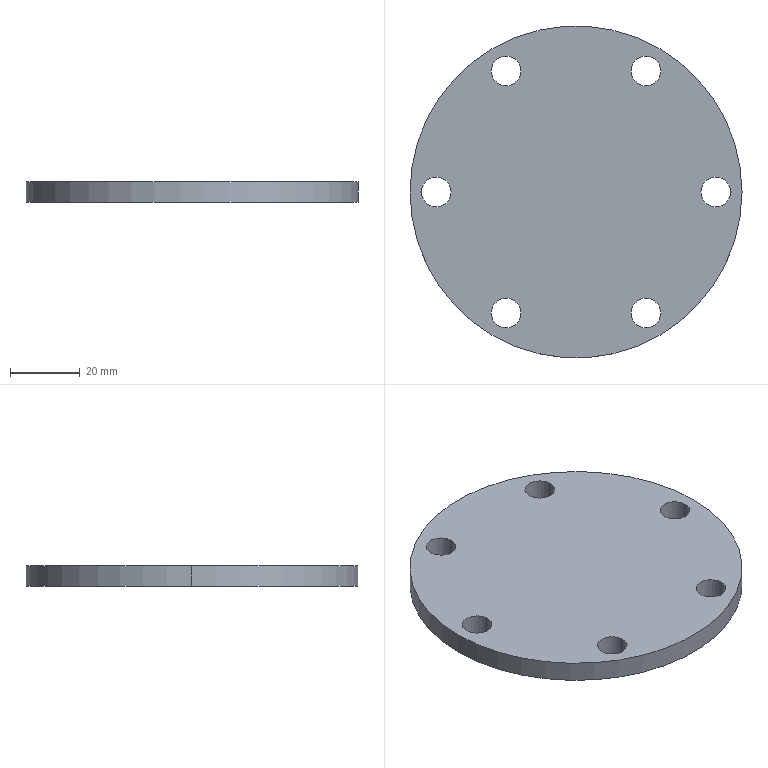Part | SolidWorks | features FlatPattern 1, SMBaseFlange 1, SheetMetal 1 | 1 solid | 16 faces | box 95 x 95 x 6 mm | volume 40486 mm3 | cylinder 14 | plane 2 | commonest cylinder face diameters 8.5 x12 95 x2
STEP:
#1=CARTESIAN_POINT('',(15.75,-34.641,6.));
#2=VERTEX_POINT('',#1);
#3=CARTESIAN_POINT('',(24.25,-34.641,6.));
#4=VERTEX_POINT('',#3);
#5=CARTESIAN_POINT('',(20.,-34.641,6.));
#6=DIRECTION('',(0.,0.,1.));
#7=DIRECTION('',(1.,0.,0.));
#8=AXIS2_PLACEMENT_3D('',#5,#6,#7);
#9=CIRCLE('',#8,4.25);
#10=EDGE_CURVE('',#2,#4,#9,.T.);
#11=ORIENTED_EDGE('',*,*,#10,.T.);
#12=CARTESIAN_POINT('',(24.25,-34.641,0.));
#13=VERTEX_POINT('',#12);
#14=CARTESIAN_POINT('',(24.25,-34.641,6.));
#15=DIRECTION('',(0.,0.,-1.));
#16=VECTOR('',#15,1000.);
#17=LINE('',#14,#16);
#18=EDGE_CURVE('',#4,#13,#17,.T.);
#19=ORIENTED_EDGE('',*,*,#18,.T.);
#20=CARTESIAN_POINT('',(15.75,-34.641,0.));
#21=VERTEX_POINT('',#20);
#22=CARTESIAN_POINT('',(20.,-34.641,0.));
#23=DIRECTION('',(0.,0.,1.));
#24=DIRECTION('',(1.,0.,0.));
#25=AXIS2_PLACEMENT_3D('',#22,#23,#24);
#26=CIRCLE('',#25,4.25);
#27=EDGE_CURVE('',#21,#13,#26,.T.);
#28=ORIENTED_EDGE('',*,*,#27,.F.);
#29=CARTESIAN_POINT('',(15.75,-34.641,6.));
#30=DIRECTION('',(0.,0.,-1.));
#31=VECTOR('',#30,1000.);
#32=LINE('',#29,#31);
#33=EDGE_CURVE('',#2,#21,#32,.T.);
#34=ORIENTED_EDGE('',*,*,#33,.F.);
#35=EDGE_LOOP('',(#11,#19,#28,#34));
#36=FACE_OUTER_BOUND('',#35,.T.);
#37=CARTESIAN_POINT('',(20.,-34.641,6.));
#38=DIRECTION('',(0.,0.,-1.));
#39=DIRECTION('',(-1.,0.,0.));
#40=AXIS2_PLACEMENT_3D('',#37,#38,#39);
#41=CYLINDRICAL_SURFACE('',#40,4.25);
#42=ADVANCED_FACE('',(#36),#41,.F.);
#43=CARTESIAN_POINT('',(35.75,0.,6.));
#44=VERTEX_POINT('',#43);
#45=CARTESIAN_POINT('',(44.25,0.,6.));
#46=VERTEX_POINT('',#45);
#47=CARTESIAN_POINT('',(40.,0.,6.));
#48=DIRECTION('',(0.,0.,1.));
#49=DIRECTION('',(1.,0.,0.));
#50=AXIS2_PLACEMENT_3D('',#47,#48,#49);
#51=CIRCLE('',#50,4.25);
#52=EDGE_CURVE('',#44,#46,#51,.T.);
#53=ORIENTED_EDGE('',*,*,#52,.T.);
#54=CARTESIAN_POINT('',(44.25,0.,0.));
#55=VERTEX_POINT('',#54);
#56=CARTESIAN_POINT('',(44.25,0.,6.));
#57=DIRECTION('',(0.,0.,-1.));
#58=VECTOR('',#57,1000.);
#59=LINE('',#56,#58);
#60=EDGE_CURVE('',#46,#55,#59,.T.);
#61=ORIENTED_EDGE('',*,*,#60,.T.);
#62=CARTESIAN_POINT('',(35.75,0.,0.));
#63=VERTEX_POINT('',#62);
#64=CARTESIAN_POINT('',(40.,0.,0.));
#65=DIRECTION('',(0.,0.,1.));
#66=DIRECTION('',(1.,0.,0.));
#67=AXIS2_PLACEMENT_3D('',#64,#65,#66);
#68=CIRCLE('',#67,4.25);
#69=EDGE_CURVE('',#63,#55,#68,.T.);
#70=ORIENTED_EDGE('',*,*,#69,.F.);
#71=CARTESIAN_POINT('',(35.75,0.,6.));
#72=DIRECTION('',(0.,0.,-1.));
#73=VECTOR('',#72,1000.);
#74=LINE('',#71,#73);
#75=EDGE_CURVE('',#44,#63,#74,.T.);
#76=ORIENTED_EDGE('',*,*,#75,.F.);
#77=EDGE_LOOP('',(#53,#61,#70,#76));
#78=FACE_OUTER_BOUND('',#77,.T.);
#79=CARTESIAN_POINT('',(40.,0.,6.));
#80=DIRECTION('',(0.,0.,-1.));
#81=DIRECTION('',(-1.,0.,0.));
#82=AXIS2_PLACEMENT_3D('',#79,#80,#81);
#83=CYLINDRICAL_SURFACE('',#82,4.25);
#84=ADVANCED_FACE('',(#78),#83,.F.);
#85=CARTESIAN_POINT('',(15.75,34.641,6.));
#86=VERTEX_POINT('',#85);
#87=CARTESIAN_POINT('',(24.25,34.641,6.));
#88=VERTEX_POINT('',#87);
#89=CARTESIAN_POINT('',(20.,34.641,6.));
#90=DIRECTION('',(0.,0.,1.));
#91=DIRECTION('',(1.,0.,0.));
#92=AXIS2_PLACEMENT_3D('',#89,#90,#91);
#93=CIRCLE('',#92,4.25);
#94=EDGE_CURVE('',#86,#88,#93,.T.);
#95=ORIENTED_EDGE('',*,*,#94,.T.);
#96=CARTESIAN_POINT('',(24.25,34.641,0.));
#97=VERTEX_POINT('',#96);
#98=CARTESIAN_POINT('',(24.25,34.641,6.));
#99=DIRECTION('',(0.,0.,-1.));
#100=VECTOR('',#99,1000.);
#101=LINE('',#98,#100);
#102=EDGE_CURVE('',#88,#97,#101,.T.);
#103=ORIENTED_EDGE('',*,*,#102,.T.);
#104=CARTESIAN_POINT('',(15.75,34.641,0.));
#105=VERTEX_POINT('',#104);
#106=CARTESIAN_POINT('',(20.,34.641,0.));
#107=DIRECTION('',(0.,0.,1.));
#108=DIRECTION('',(1.,0.,0.));
#109=AXIS2_PLACEMENT_3D('',#106,#107,#108);
#110=CIRCLE('',#109,4.25);
#111=EDGE_CURVE('',#105,#97,#110,.T.);
#112=ORIENTED_EDGE('',*,*,#111,.F.);
#113=CARTESIAN_POINT('',(15.75,34.641,6.));
#114=DIRECTION('',(0.,0.,-1.));
#115=VECTOR('',#114,1000.);
#116=LINE('',#113,#115);
#117=EDGE_CURVE('',#86,#105,#116,.T.);
#118=ORIENTED_EDGE('',*,*,#117,.F.);
#119=EDGE_LOOP('',(#95,#103,#112,#118));
#120=FACE_OUTER_BOUND('',#119,.T.);
#121=CARTESIAN_POINT('',(20.,34.641,6.));
#122=DIRECTION('',(0.,0.,-1.));
#123=DIRECTION('',(-1.,0.,0.));
#124=AXIS2_PLACEMENT_3D('',#121,#122,#123);
#125=CYLINDRICAL_SURFACE('',#124,4.25);
#126=ADVANCED_FACE('',(#120),#125,.F.);
#127=CARTESIAN_POINT('',(-24.25,34.641,6.));
#128=VERTEX_POINT('',#127);
#129=CARTESIAN_POINT('',(-15.75,34.641,6.));
#130=VERTEX_POINT('',#129);
#131=CARTESIAN_POINT('',(-20.,34.641,6.));
#132=DIRECTION('',(0.,0.,1.));
#133=DIRECTION('',(1.,0.,0.));
#134=AXIS2_PLACEMENT_3D('',#131,#132,#133);
#135=CIRCLE('',#134,4.25);
#136=EDGE_CURVE('',#128,#130,#135,.T.);
#137=ORIENTED_EDGE('',*,*,#136,.T.);
#138=CARTESIAN_POINT('',(-15.75,34.641,0.));
#139=VERTEX_POINT('',#138);
#140=CARTESIAN_POINT('',(-15.75,34.641,6.));
#141=DIRECTION('',(0.,0.,-1.));
#142=VECTOR('',#141,1000.);
#143=LINE('',#140,#142);
#144=EDGE_CURVE('',#130,#139,#143,.T.);
#145=ORIENTED_EDGE('',*,*,#144,.T.);
#146=CARTESIAN_POINT('',(-24.25,34.641,0.));
#147=VERTEX_POINT('',#146);
#148=CARTESIAN_POINT('',(-20.,34.641,0.));
#149=DIRECTION('',(0.,0.,1.));
#150=DIRECTION('',(1.,0.,0.));
#151=AXIS2_PLACEMENT_3D('',#148,#149,#150);
#152=CIRCLE('',#151,4.25);
#153=EDGE_CURVE('',#147,#139,#152,.T.);
#154=ORIENTED_EDGE('',*,*,#153,.F.);
#155=CARTESIAN_POINT('',(-24.25,34.641,6.));
#156=DIRECTION('',(0.,0.,-1.));
#157=VECTOR('',#156,1000.);
#158=LINE('',#155,#157);
#159=EDGE_CURVE('',#128,#147,#158,.T.);
#160=ORIENTED_EDGE('',*,*,#159,.F.);
#161=EDGE_LOOP('',(#137,#145,#154,#160));
#162=FACE_OUTER_BOUND('',#161,.T.);
#163=CARTESIAN_POINT('',(-20.,34.641,6.));
#164=DIRECTION('',(0.,0.,-1.));
#165=DIRECTION('',(-1.,0.,0.));
#166=AXIS2_PLACEMENT_3D('',#163,#164,#165);
#167=CYLINDRICAL_SURFACE('',#166,4.25);
#168=ADVANCED_FACE('',(#162),#167,.F.);
#169=CARTESIAN_POINT('',(-44.25,0.,6.));
#170=VERTEX_POINT('',#169);
#171=CARTESIAN_POINT('',(-35.75,0.,6.));
#172=VERTEX_POINT('',#171);
#173=CARTESIAN_POINT('',(-40.,0.,6.));
#174=DIRECTION('',(0.,0.,1.));
#175=DIRECTION('',(1.,0.,0.));
#176=AXIS2_PLACEMENT_3D('',#173,#174,#175);
#177=CIRCLE('',#176,4.25);
#178=EDGE_CURVE('',#170,#172,#177,.T.);
#179=ORIENTED_EDGE('',*,*,#178,.T.);
#180=CARTESIAN_POINT('',(-35.75,0.,0.));
#181=VERTEX_POINT('',#180);
#182=CARTESIAN_POINT('',(-35.75,0.,6.));
#183=DIRECTION('',(0.,0.,-1.));
#184=VECTOR('',#183,1000.);
#185=LINE('',#182,#184);
#186=EDGE_CURVE('',#172,#181,#185,.T.);
#187=ORIENTED_EDGE('',*,*,#186,.T.);
#188=CARTESIAN_POINT('',(-44.25,0.,0.));
#189=VERTEX_POINT('',#188);
#190=CARTESIAN_POINT('',(-40.,0.,0.));
#191=DIRECTION('',(0.,0.,1.));
#192=DIRECTION('',(1.,0.,0.));
#193=AXIS2_PLACEMENT_3D('',#190,#191,#192);
#194=CIRCLE('',#193,4.25);
#195=EDGE_CURVE('',#189,#181,#194,.T.);
#196=ORIENTED_EDGE('',*,*,#195,.F.);
#197=CARTESIAN_POINT('',(-44.25,0.,6.));
#198=DIRECTION('',(0.,0.,-1.));
#199=VECTOR('',#198,1000.);
#200=LINE('',#197,#199);
#201=EDGE_CURVE('',#170,#189,#200,.T.);
#202=ORIENTED_EDGE('',*,*,#201,.F.);
#203=EDGE_LOOP('',(#179,#187,#196,#202));
#204=FACE_OUTER_BOUND('',#203,.T.);
#205=CARTESIAN_POINT('',(-40.,0.,6.));
#206=DIRECTION('',(0.,0.,-1.));
#207=DIRECTION('',(-1.,0.,0.));
#208=AXIS2_PLACEMENT_3D('',#205,#206,#207);
#209=CYLINDRICAL_SURFACE('',#208,4.25);
#210=ADVANCED_FACE('',(#204),#209,.F.);
#211=CARTESIAN_POINT('',(-24.25,-34.641,6.));
#212=VERTEX_POINT('',#211);
#213=CARTESIAN_POINT('',(-15.75,-34.641,6.));
#214=VERTEX_POINT('',#213);
#215=CARTESIAN_POINT('',(-20.,-34.641,6.));
#216=DIRECTION('',(0.,0.,1.));
#217=DIRECTION('',(1.,0.,0.));
#218=AXIS2_PLACEMENT_3D('',#215,#216,#217);
#219=CIRCLE('',#218,4.25);
#220=EDGE_CURVE('',#212,#214,#219,.T.);
#221=ORIENTED_EDGE('',*,*,#220,.T.);
#222=CARTESIAN_POINT('',(-15.75,-34.641,0.));
#223=VERTEX_POINT('',#222);
#224=CARTESIAN_POINT('',(-15.75,-34.641,6.));
#225=DIRECTION('',(0.,0.,-1.));
#226=VECTOR('',#225,1000.);
#227=LINE('',#224,#226);
#228=EDGE_CURVE('',#214,#223,#227,.T.);
#229=ORIENTED_EDGE('',*,*,#228,.T.);
#230=CARTESIAN_POINT('',(-24.25,-34.641,0.));
#231=VERTEX_POINT('',#230);
#232=CARTESIAN_POINT('',(-20.,-34.641,0.));
#233=DIRECTION('',(0.,0.,1.));
#234=DIRECTION('',(1.,0.,0.));
#235=AXIS2_PLACEMENT_3D('',#232,#233,#234);
#236=CIRCLE('',#235,4.25);
#237=EDGE_CURVE('',#231,#223,#236,.T.);
#238=ORIENTED_EDGE('',*,*,#237,.F.);
#239=CARTESIAN_POINT('',(-24.25,-34.641,6.));
#240=DIRECTION('',(0.,0.,-1.));
#241=VECTOR('',#240,1000.);
#242=LINE('',#239,#241);
#243=EDGE_CURVE('',#212,#231,#242,.T.);
#244=ORIENTED_EDGE('',*,*,#243,.F.);
#245=EDGE_LOOP('',(#221,#229,#238,#244));
#246=FACE_OUTER_BOUND('',#245,.T.);
#247=CARTESIAN_POINT('',(-20.,-34.641,6.));
#248=DIRECTION('',(0.,0.,-1.));
#249=DIRECTION('',(-1.,0.,0.));
#250=AXIS2_PLACEMENT_3D('',#247,#248,#249);
#251=CYLINDRICAL_SURFACE('',#250,4.25);
#252=ADVANCED_FACE('',(#246),#251,.F.);
#253=CARTESIAN_POINT('',(47.5,0.,6.));
#254=VERTEX_POINT('',#253);
#255=CARTESIAN_POINT('',(-47.5,0.,6.));
#256=VERTEX_POINT('',#255);
#257=CARTESIAN_POINT('',(0.,0.,6.));
#258=DIRECTION('',(0.,0.,1.));
#259=DIRECTION('',(1.,0.,0.));
#260=AXIS2_PLACEMENT_3D('',#257,#258,#259);
#261=CIRCLE('',#260,47.5);
#262=EDGE_CURVE('',#254,#256,#261,.T.);
#263=ORIENTED_EDGE('',*,*,#262,.F.);
#264=CARTESIAN_POINT('',(47.5,0.,0.));
#265=VERTEX_POINT('',#264);
#266=CARTESIAN_POINT('',(47.5,0.,6.));
#267=DIRECTION('',(0.,0.,-1.));
#268=VECTOR('',#267,1000.);
#269=LINE('',#266,#268);
#270=EDGE_CURVE('',#254,#265,#269,.T.);
#271=ORIENTED_EDGE('',*,*,#270,.T.);
#272=CARTESIAN_POINT('',(-47.5,0.,0.));
#273=VERTEX_POINT('',#272);
#274=CARTESIAN_POINT('',(0.,0.,0.));
#275=DIRECTION('',(0.,0.,1.));
#276=DIRECTION('',(1.,0.,0.));
#277=AXIS2_PLACEMENT_3D('',#274,#275,#276);
#278=CIRCLE('',#277,47.5);
#279=EDGE_CURVE('',#265,#273,#278,.T.);
#280=ORIENTED_EDGE('',*,*,#279,.T.);
#281=CARTESIAN_POINT('',(-47.5,0.,6.));
#282=DIRECTION('',(0.,0.,-1.));
#283=VECTOR('',#282,1000.);
#284=LINE('',#281,#283);
#285=EDGE_CURVE('',#256,#273,#284,.T.);
#286=ORIENTED_EDGE('',*,*,#285,.F.);
#287=EDGE_LOOP('',(#263,#271,#280,#286));
#288=FACE_OUTER_BOUND('',#287,.T.);
#289=CARTESIAN_POINT('',(0.,0.,6.));
#290=DIRECTION('',(0.,0.,-1.));
#291=DIRECTION('',(-1.,0.,0.));
#292=AXIS2_PLACEMENT_3D('',#289,#290,#291);
#293=CYLINDRICAL_SURFACE('',#292,47.5);
#294=ADVANCED_FACE('',(#288),#293,.T.);
#295=ORIENTED_EDGE('',*,*,#52,.F.);
#296=CARTESIAN_POINT('',(40.,0.,6.));
#297=DIRECTION('',(0.,0.,1.));
#298=DIRECTION('',(1.,0.,0.));
#299=AXIS2_PLACEMENT_3D('',#296,#297,#298);
#300=CIRCLE('',#299,4.25);
#301=EDGE_CURVE('',#46,#44,#300,.T.);
#302=ORIENTED_EDGE('',*,*,#301,.F.);
#303=EDGE_LOOP('',(#295,#302));
#304=FACE_BOUND('',#303,.T.);
#305=ORIENTED_EDGE('',*,*,#136,.F.);
#306=CARTESIAN_POINT('',(-20.,34.641,6.));
#307=DIRECTION('',(0.,0.,1.));
#308=DIRECTION('',(1.,0.,0.));
#309=AXIS2_PLACEMENT_3D('',#306,#307,#308);
#310=CIRCLE('',#309,4.25);
#311=EDGE_CURVE('',#130,#128,#310,.T.);
#312=ORIENTED_EDGE('',*,*,#311,.F.);
#313=EDGE_LOOP('',(#305,#312));
#314=FACE_BOUND('',#313,.T.);
#315=ORIENTED_EDGE('',*,*,#220,.F.);
#316=CARTESIAN_POINT('',(-20.,-34.641,6.));
#317=DIRECTION('',(0.,0.,1.));
#318=DIRECTION('',(1.,0.,0.));
#319=AXIS2_PLACEMENT_3D('',#316,#317,#318);
#320=CIRCLE('',#319,4.25);
#321=EDGE_CURVE('',#214,#212,#320,.T.);
#322=ORIENTED_EDGE('',*,*,#321,.F.);
#323=EDGE_LOOP('',(#315,#322));
#324=FACE_BOUND('',#323,.T.);
#325=CARTESIAN_POINT('',(0.,0.,6.));
#326=DIRECTION('',(0.,0.,1.));
#327=DIRECTION('',(1.,0.,0.));
#328=AXIS2_PLACEMENT_3D('',#325,#326,#327);
#329=CIRCLE('',#328,47.5);
#330=EDGE_CURVE('',#256,#254,#329,.T.);
#331=ORIENTED_EDGE('',*,*,#330,.T.);
#332=ORIENTED_EDGE('',*,*,#262,.T.);
#333=EDGE_LOOP('',(#331,#332));
#334=FACE_OUTER_BOUND('',#333,.T.);
#335=ORIENTED_EDGE('',*,*,#178,.F.);
#336=CARTESIAN_POINT('',(-40.,0.,6.));
#337=DIRECTION('',(0.,0.,1.));
#338=DIRECTION('',(1.,0.,0.));
#339=AXIS2_PLACEMENT_3D('',#336,#337,#338);
#340=CIRCLE('',#339,4.25);
#341=EDGE_CURVE('',#172,#170,#340,.T.);
#342=ORIENTED_EDGE('',*,*,#341,.F.);
#343=EDGE_LOOP('',(#335,#342));
#344=FACE_BOUND('',#343,.T.);
#345=ORIENTED_EDGE('',*,*,#94,.F.);
#346=CARTESIAN_POINT('',(20.,34.641,6.));
#347=DIRECTION('',(0.,0.,1.));
#348=DIRECTION('',(1.,0.,0.));
#349=AXIS2_PLACEMENT_3D('',#346,#347,#348);
#350=CIRCLE('',#349,4.25);
#351=EDGE_CURVE('',#88,#86,#350,.T.);
#352=ORIENTED_EDGE('',*,*,#351,.F.);
#353=EDGE_LOOP('',(#345,#352));
#354=FACE_BOUND('',#353,.T.);
#355=ORIENTED_EDGE('',*,*,#10,.F.);
#356=CARTESIAN_POINT('',(20.,-34.641,6.));
#357=DIRECTION('',(0.,0.,1.));
#358=DIRECTION('',(1.,0.,0.));
#359=AXIS2_PLACEMENT_3D('',#356,#357,#358);
#360=CIRCLE('',#359,4.25);
#361=EDGE_CURVE('',#4,#2,#360,.T.);
#362=ORIENTED_EDGE('',*,*,#361,.F.);
#363=EDGE_LOOP('',(#355,#362));
#364=FACE_BOUND('',#363,.T.);
#365=CARTESIAN_POINT('',(0.,0.,6.));
#366=DIRECTION('',(0.,0.,1.));
#367=DIRECTION('',(1.,0.,0.));
#368=AXIS2_PLACEMENT_3D('',#365,#366,#367);
#369=PLANE('',#368);
#370=ADVANCED_FACE('',(#304,#314,#324,#334,#344,#354,#364),#369,.T.);
#371=CARTESIAN_POINT('',(0.,0.,0.));
#372=DIRECTION('',(0.,0.,1.));
#373=DIRECTION('',(1.,0.,0.));
#374=AXIS2_PLACEMENT_3D('',#371,#372,#373);
#375=CIRCLE('',#374,47.5);
#376=EDGE_CURVE('',#273,#265,#375,.T.);
#377=ORIENTED_EDGE('',*,*,#376,.F.);
#378=ORIENTED_EDGE('',*,*,#279,.F.);
#379=EDGE_LOOP('',(#377,#378));
#380=FACE_OUTER_BOUND('',#379,.T.);
#381=ORIENTED_EDGE('',*,*,#237,.T.);
#382=CARTESIAN_POINT('',(-20.,-34.641,0.));
#383=DIRECTION('',(0.,0.,1.));
#384=DIRECTION('',(1.,0.,0.));
#385=AXIS2_PLACEMENT_3D('',#382,#383,#384);
#386=CIRCLE('',#385,4.25);
#387=EDGE_CURVE('',#223,#231,#386,.T.);
#388=ORIENTED_EDGE('',*,*,#387,.T.);
#389=EDGE_LOOP('',(#381,#388));
#390=FACE_BOUND('',#389,.T.);
#391=ORIENTED_EDGE('',*,*,#195,.T.);
#392=CARTESIAN_POINT('',(-40.,0.,0.));
#393=DIRECTION('',(0.,0.,1.));
#394=DIRECTION('',(1.,0.,0.));
#395=AXIS2_PLACEMENT_3D('',#392,#393,#394);
#396=CIRCLE('',#395,4.25);
#397=EDGE_CURVE('',#181,#189,#396,.T.);
#398=ORIENTED_EDGE('',*,*,#397,.T.);
#399=EDGE_LOOP('',(#391,#398));
#400=FACE_BOUND('',#399,.T.);
#401=ORIENTED_EDGE('',*,*,#153,.T.);
#402=CARTESIAN_POINT('',(-20.,34.641,0.));
#403=DIRECTION('',(0.,0.,1.));
#404=DIRECTION('',(1.,0.,0.));
#405=AXIS2_PLACEMENT_3D('',#402,#403,#404);
#406=CIRCLE('',#405,4.25);
#407=EDGE_CURVE('',#139,#147,#406,.T.);
#408=ORIENTED_EDGE('',*,*,#407,.T.);
#409=EDGE_LOOP('',(#401,#408));
#410=FACE_BOUND('',#409,.T.);
#411=ORIENTED_EDGE('',*,*,#111,.T.);
#412=CARTESIAN_POINT('',(20.,34.641,0.));
#413=DIRECTION('',(0.,0.,1.));
#414=DIRECTION('',(1.,0.,0.));
#415=AXIS2_PLACEMENT_3D('',#412,#413,#414);
#416=CIRCLE('',#415,4.25);
#417=EDGE_CURVE('',#97,#105,#416,.T.);
#418=ORIENTED_EDGE('',*,*,#417,.T.);
#419=EDGE_LOOP('',(#411,#418));
#420=FACE_BOUND('',#419,.T.);
#421=ORIENTED_EDGE('',*,*,#69,.T.);
#422=CARTESIAN_POINT('',(40.,0.,0.));
#423=DIRECTION('',(0.,0.,1.));
#424=DIRECTION('',(1.,0.,0.));
#425=AXIS2_PLACEMENT_3D('',#422,#423,#424);
#426=CIRCLE('',#425,4.25);
#427=EDGE_CURVE('',#55,#63,#426,.T.);
#428=ORIENTED_EDGE('',*,*,#427,.T.);
#429=EDGE_LOOP('',(#421,#428));
#430=FACE_BOUND('',#429,.T.);
#431=ORIENTED_EDGE('',*,*,#27,.T.);
#432=CARTESIAN_POINT('',(20.,-34.641,0.));
#433=DIRECTION('',(0.,0.,1.));
#434=DIRECTION('',(1.,0.,0.));
#435=AXIS2_PLACEMENT_3D('',#432,#433,#434);
#436=CIRCLE('',#435,4.25);
#437=EDGE_CURVE('',#13,#21,#436,.T.);
#438=ORIENTED_EDGE('',*,*,#437,.T.);
#439=EDGE_LOOP('',(#431,#438));
#440=FACE_BOUND('',#439,.T.);
#441=CARTESIAN_POINT('',(0.,0.,0.));
#442=DIRECTION('',(0.,0.,1.));
#443=DIRECTION('',(1.,0.,0.));
#444=AXIS2_PLACEMENT_3D('',#441,#442,#443);
#445=PLANE('',#444);
#446=ADVANCED_FACE('',(#380,#390,#400,#410,#420,#430,#440),#445,.F.);
#447=ORIENTED_EDGE('',*,*,#270,.F.);
#448=ORIENTED_EDGE('',*,*,#330,.F.);
#449=ORIENTED_EDGE('',*,*,#285,.T.);
#450=ORIENTED_EDGE('',*,*,#376,.T.);
#451=EDGE_LOOP('',(#447,#448,#449,#450));
#452=FACE_OUTER_BOUND('',#451,.T.);
#453=CARTESIAN_POINT('',(0.,0.,6.));
#454=DIRECTION('',(0.,0.,-1.));
#455=DIRECTION('',(-1.,0.,0.));
#456=AXIS2_PLACEMENT_3D('',#453,#454,#455);
#457=CYLINDRICAL_SURFACE('',#456,47.5);
#458=ADVANCED_FACE('',(#452),#457,.T.);
#459=ORIENTED_EDGE('',*,*,#228,.F.);
#460=ORIENTED_EDGE('',*,*,#321,.T.);
#461=ORIENTED_EDGE('',*,*,#243,.T.);
#462=ORIENTED_EDGE('',*,*,#387,.F.);
#463=EDGE_LOOP('',(#459,#460,#461,#462));
#464=FACE_OUTER_BOUND('',#463,.T.);
#465=CARTESIAN_POINT('',(-20.,-34.641,6.));
#466=DIRECTION('',(0.,0.,-1.));
#467=DIRECTION('',(-1.,0.,0.));
#468=AXIS2_PLACEMENT_3D('',#465,#466,#467);
#469=CYLINDRICAL_SURFACE('',#468,4.25);
#470=ADVANCED_FACE('',(#464),#469,.F.);
#471=ORIENTED_EDGE('',*,*,#186,.F.);
#472=ORIENTED_EDGE('',*,*,#341,.T.);
#473=ORIENTED_EDGE('',*,*,#201,.T.);
#474=ORIENTED_EDGE('',*,*,#397,.F.);
#475=EDGE_LOOP('',(#471,#472,#473,#474));
#476=FACE_OUTER_BOUND('',#475,.T.);
#477=CARTESIAN_POINT('',(-40.,0.,6.));
#478=DIRECTION('',(0.,0.,-1.));
#479=DIRECTION('',(-1.,0.,0.));
#480=AXIS2_PLACEMENT_3D('',#477,#478,#479);
#481=CYLINDRICAL_SURFACE('',#480,4.25);
#482=ADVANCED_FACE('',(#476),#481,.F.);
#483=ORIENTED_EDGE('',*,*,#144,.F.);
#484=ORIENTED_EDGE('',*,*,#311,.T.);
#485=ORIENTED_EDGE('',*,*,#159,.T.);
#486=ORIENTED_EDGE('',*,*,#407,.F.);
#487=EDGE_LOOP('',(#483,#484,#485,#486));
#488=FACE_OUTER_BOUND('',#487,.T.);
#489=CARTESIAN_POINT('',(-20.,34.641,6.));
#490=DIRECTION('',(0.,0.,-1.));
#491=DIRECTION('',(-1.,0.,0.));
#492=AXIS2_PLACEMENT_3D('',#489,#490,#491);
#493=CYLINDRICAL_SURFACE('',#492,4.25);
#494=ADVANCED_FACE('',(#488),#493,.F.);
#495=ORIENTED_EDGE('',*,*,#102,.F.);
#496=ORIENTED_EDGE('',*,*,#351,.T.);
#497=ORIENTED_EDGE('',*,*,#117,.T.);
#498=ORIENTED_EDGE('',*,*,#417,.F.);
#499=EDGE_LOOP('',(#495,#496,#497,#498));
#500=FACE_OUTER_BOUND('',#499,.T.);
#501=CARTESIAN_POINT('',(20.,34.641,6.));
#502=DIRECTION('',(0.,0.,-1.));
#503=DIRECTION('',(-1.,0.,0.));
#504=AXIS2_PLACEMENT_3D('',#501,#502,#503);
#505=CYLINDRICAL_SURFACE('',#504,4.25);
#506=ADVANCED_FACE('',(#500),#505,.F.);
#507=ORIENTED_EDGE('',*,*,#60,.F.);
#508=ORIENTED_EDGE('',*,*,#301,.T.);
#509=ORIENTED_EDGE('',*,*,#75,.T.);
#510=ORIENTED_EDGE('',*,*,#427,.F.);
#511=EDGE_LOOP('',(#507,#508,#509,#510));
#512=FACE_OUTER_BOUND('',#511,.T.);
#513=CARTESIAN_POINT('',(40.,0.,6.));
#514=DIRECTION('',(0.,0.,-1.));
#515=DIRECTION('',(-1.,0.,0.));
#516=AXIS2_PLACEMENT_3D('',#513,#514,#515);
#517=CYLINDRICAL_SURFACE('',#516,4.25);
#518=ADVANCED_FACE('',(#512),#517,.F.);
#519=ORIENTED_EDGE('',*,*,#18,.F.);
#520=ORIENTED_EDGE('',*,*,#361,.T.);
#521=ORIENTED_EDGE('',*,*,#33,.T.);
#522=ORIENTED_EDGE('',*,*,#437,.F.);
#523=EDGE_LOOP('',(#519,#520,#521,#522));
#524=FACE_OUTER_BOUND('',#523,.T.);
#525=CARTESIAN_POINT('',(20.,-34.641,6.));
#526=DIRECTION('',(0.,0.,-1.));
#527=DIRECTION('',(-1.,0.,0.));
#528=AXIS2_PLACEMENT_3D('',#525,#526,#527);
#529=CYLINDRICAL_SURFACE('',#528,4.25);
#530=ADVANCED_FACE('',(#524),#529,.F.);
#531=CLOSED_SHELL('',(#42,#84,#126,#168,#210,#252,#294,#370,#446,#458,#470,#482,#494,#506,#518,#530));
#532=MANIFOLD_SOLID_BREP('',#531);
#533=CARTESIAN_POINT('',(0.,0.,0.));
#534=DIRECTION('',(0.,0.,1.));
#535=DIRECTION('',(1.,0.,0.));
#536=AXIS2_PLACEMENT_3D('',#533,#534,#535);
#537=(LENGTH_UNIT()NAMED_UNIT(*)SI_UNIT(.MILLI.,.METRE.));
#538=UNCERTAINTY_MEASURE_WITH_UNIT(LENGTH_MEASURE(0.00001),#537,'','');
#539=(NAMED_UNIT(*)PLANE_ANGLE_UNIT()SI_UNIT($,.RADIAN.));
#540=(NAMED_UNIT(*)SI_UNIT($,.STERADIAN.)SOLID_ANGLE_UNIT());
#541=(GEOMETRIC_REPRESENTATION_CONTEXT(3)GLOBAL_UNCERTAINTY_ASSIGNED_CONTEXT((#538))GLOBAL_UNIT_ASSIGNED_CONTEXT((#537,#539,#540))REPRESENTATION_CONTEXT('',''));
#542=ADVANCED_BREP_SHAPE_REPRESENTATION('',(#532,#536),#541);